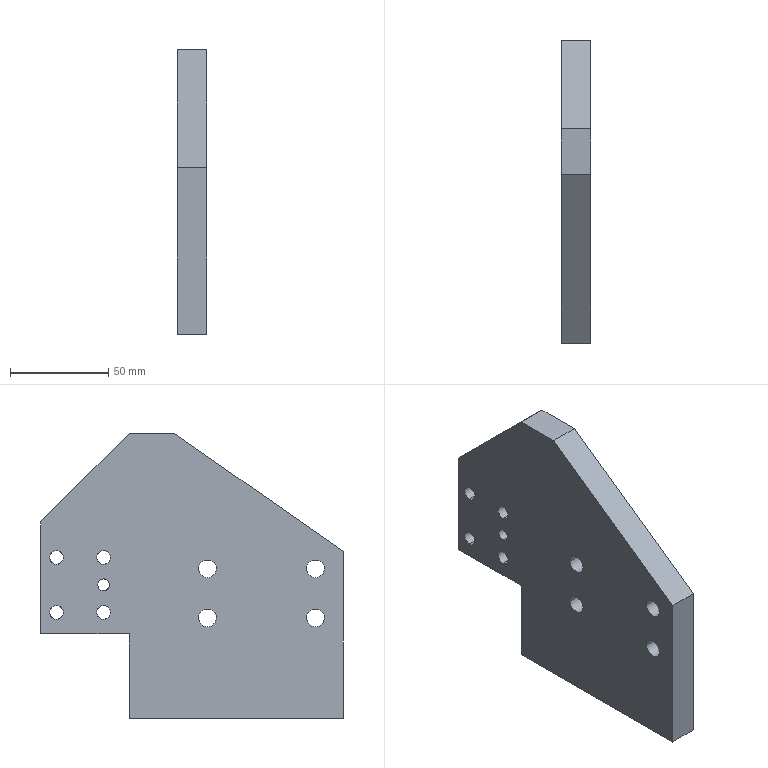Part | STEP file | Positioning_id1714_x_t | 1 solid | 28 faces | box 15 x 154 x 145 mm | volume 245583 mm3 | cylinder 18 | plane 10 | commonest cylinder face diameters 7 x8 9 x8 6 x2